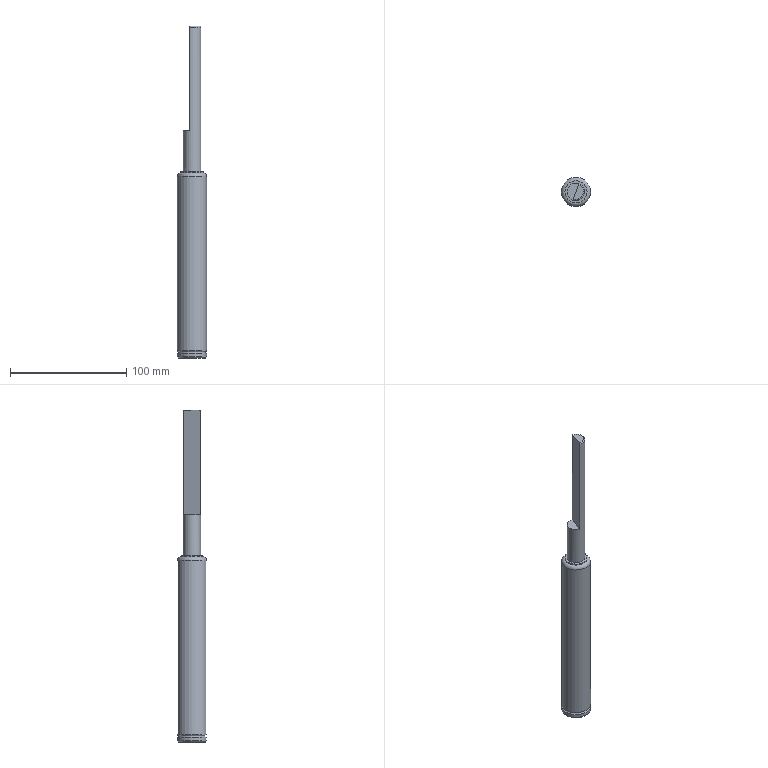Part | NX | features 24 2 | 1 solid | 87 faces | box 25 x 25 x 285 mm | volume 91972 mm3 | plane 54 | spline 22 | cylinder 6 | torus 3 | cone 2 | commonest cylinder face diameters 25 x2 5 x1 6 x1 15 x1 18.904 x1